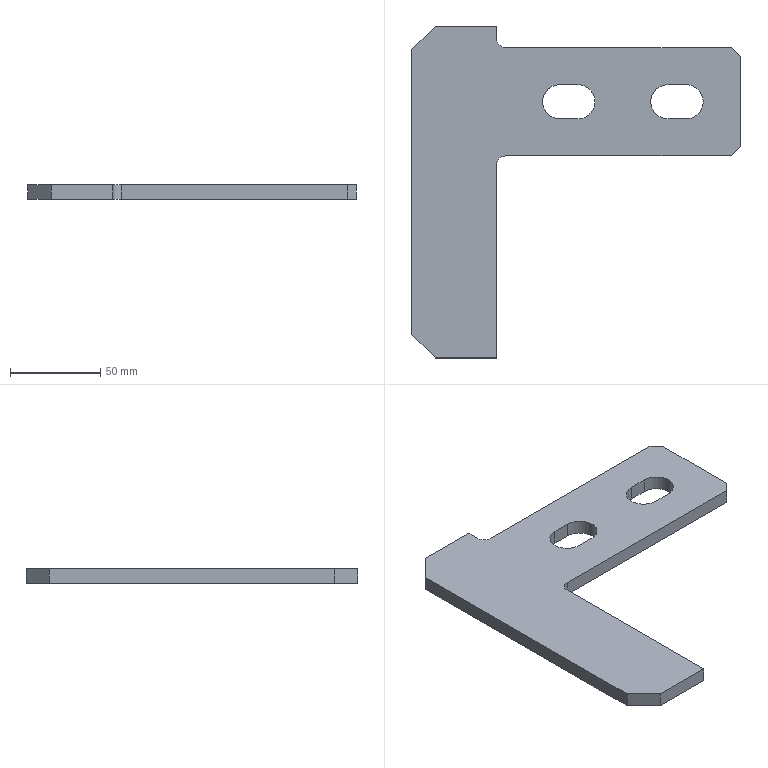Part | STEP file | 筋Plate-200×100-100 | 1 solid | 26 faces | box 182 x 184 x 8 mm | volume 124941 mm3 | plane 18 | cylinder 8 | commonest cylinder face diameters 19 x6 10 x2